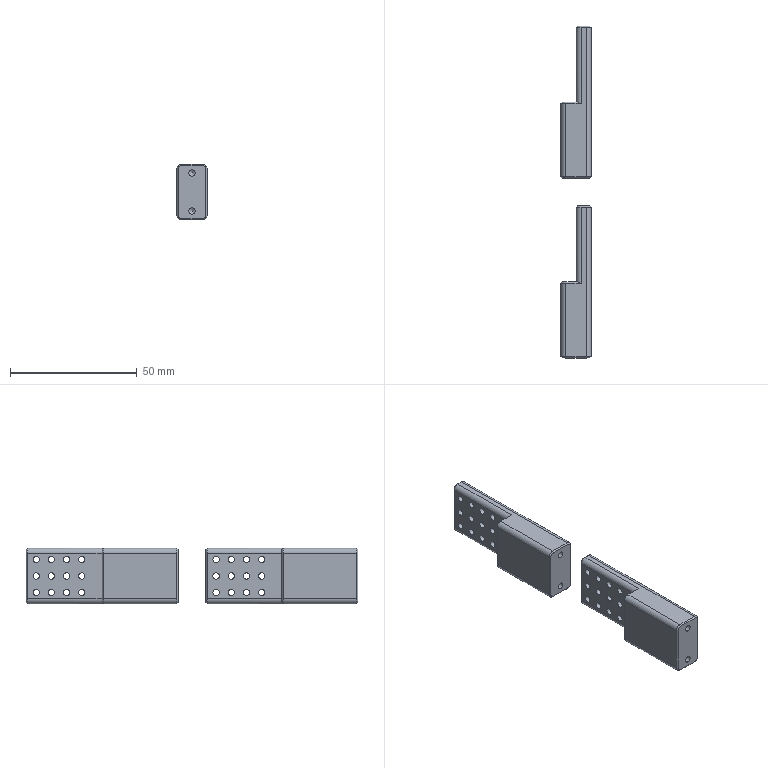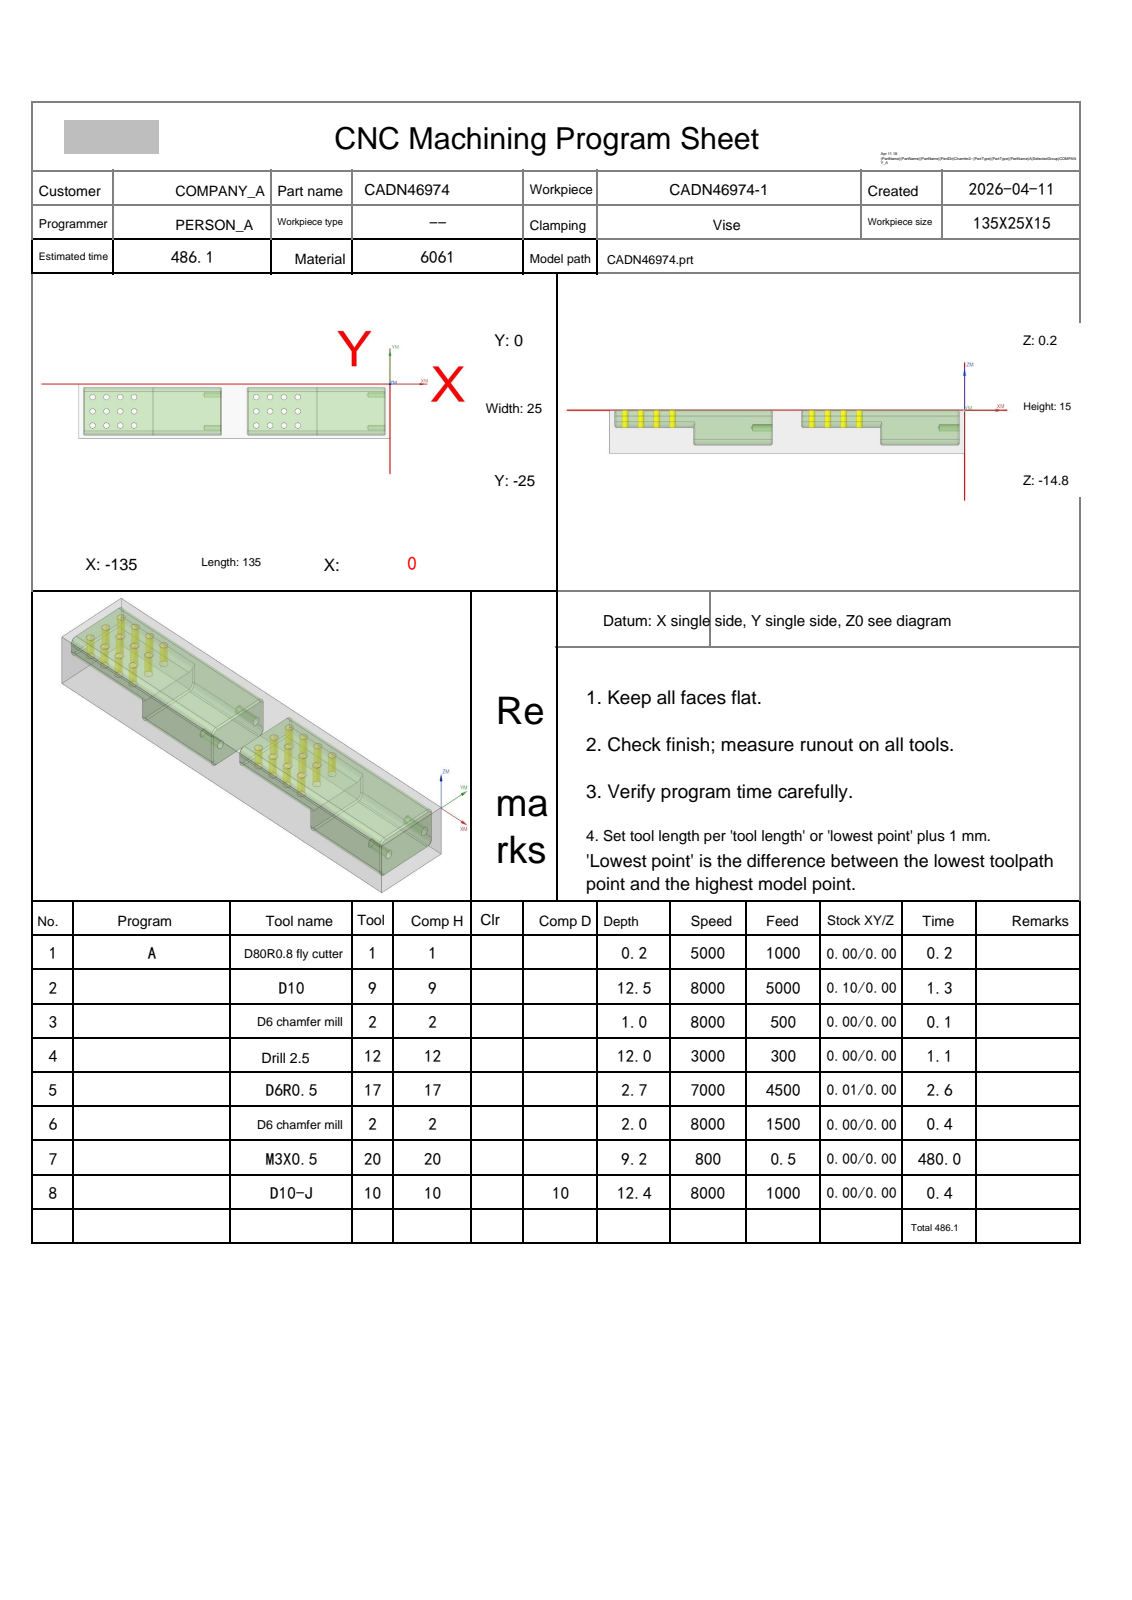NC program | NX | posted by the shop | part box 12 x 131 x 22 mm
Lines 1 to 672 of 2479:
%
O0001
(Machine time: 919.72 MIN)
(===Total Tool:7===)
(T1=D80R0.8 fly cutter D=80.  R=0.8  D-  H01 Z=0.    )
(T9=D10     D=10.  R=0.   D-  H09 Z=-12.3 )
(T2=D6 chamfer mill   D=6.   R=0.   D-  H02 Z=-1.75 )
(T12=drill 2.5  D=2.5  DR_a=118 D-  H12 Z=-11.75)
(T17=D6R0.5 D=6.   R=0.5  D-  H17 Z=-2.5  )
(T20=M3X0.5 D=2.5  DR_a=180 D-  H20 Z=-9.   )
(T10=D10-J  D=10.  R=0.   D10 H10 Z=-12.2 )
G80 G90 G17 G49 G40
G91 G28 Z0
M01
N1 T01 M06
(D80R0.8 fly cutter  D=80. R=0.8 H=01 ce=0.00 di=0.00)
G00 G90 G54 X43. Y-12.5 M03 S5000
G43 H01 Z20.
M08
Z2.
G01 Z0.0 F1000.
X38.
X-173.
X-178.
Z2.
G00 Z20.
G91 G28 Z0.0
M05
M09
G91 G28 Z0.0
M01
N2 T09 M06
(D10  D=10. R=0. H=09 ce=0.10 di=0.00)
G00 G90 G54 X-103. Y-28.6 M03 S8000
G43 H09 Z20.
M08
Z.5
G01 X-132.5 Z.379 F5000.
G02 X-136.106 Y-27.106 Z.362 I0.0 J5.1
G01 X-136.606 Y-26.606 Z.36
G02 X-138.1 Y-23. Z.343 I3.606 J3.606
G01 Y-2. Z.257
G02 X-136.606 Y1.606 Z.24 I5.1 J0.0
G01 X-136.106 Y2.106 Z.238
G02 X-132.5 Y3.6 Z.221 I3.606 J-3.606
G01 X-73.5 Z-.021
G02 X-69.894 Y2.106 Z-.038 I0.0 J-5.1
G01 X-69.394 Y1.606 Z-.04
G02 X-67.9 Y-2. Z-.057 I-3.606 J-3.606
G01 Y-23. Z-.143
G02 X-69.394 Y-26.606 Z-.16 I-5.1 J0.0
G01 X-69.894 Y-27.106 Z-.162
G02 X-73.5 Y-28.6 Z-.179 I-3.606 J3.606
G01 X-132.5 Z-.421
G02 X-136.106 Y-27.106 Z-.438 I0.0 J5.1
G01 X-136.606 Y-26.606 Z-.44
G02 X-138.1 Y-23. Z-.457 I3.606 J3.606
G01 Y-2. Z-.543
G02 X-136.606 Y1.606 Z-.56 I5.1 J0.0
G01 X-136.106 Y2.106 Z-.562
G02 X-132.5 Y3.6 Z-.579 I3.606 J-3.606
G01 X-73.5 Z-.821
G02 X-69.894 Y2.106 Z-.838 I0.0 J-5.1
G01 X-69.394 Y1.606 Z-.84
G02 X-67.9 Y-2. Z-.857 I-3.606 J-3.606
G01 Y-23. Z-.943
G02 X-69.394 Y-26.606 Z-.96 I-5.1 J0.0
G01 X-69.894 Y-27.106 Z-.962
G02 X-73.5 Y-28.6 Z-.979 I-3.606 J3.606
G01 X-132.5 Z-1.221
G02 X-136.106 Y-27.106 Z-1.238 I0.0 J5.1
G01 X-136.606 Y-26.606 Z-1.24
G02 X-138.1 Y-23. Z-1.257 I3.606 J3.606
G01 Y-2. Z-1.343
G02 X-136.606 Y1.606 Z-1.36 I5.1 J0.0
G01 X-136.106 Y2.106 Z-1.362
G02 X-132.5 Y3.6 Z-1.379 I3.606 J-3.606
G01 X-73.5 Z-1.621
G02 X-69.894 Y2.106 Z-1.638 I0.0 J-5.1
G01 X-69.394 Y1.606 Z-1.64
G02 X-67.9 Y-2. Z-1.657 I-3.606 J-3.606
G01 Y-23. Z-1.743
G02 X-69.394 Y-26.606 Z-1.76 I-5.1 J0.0
G01 X-69.894 Y-27.106 Z-1.762
G02 X-73.5 Y-28.6 Z-1.779 I-3.606 J3.606
G01 X-132.5 Z-2.021
G02 X-136.106 Y-27.106 Z-2.038 I0.0 J5.1
G01 X-136.606 Y-26.606 Z-2.04
G02 X-138.1 Y-23. Z-2.057 I3.606 J3.606
G01 Y-2. Z-2.143
G02 X-136.606 Y1.606 Z-2.16 I5.1 J0.0
G01 X-136.106 Y2.106 Z-2.162
G02 X-132.5 Y3.6 Z-2.179 I3.606 J-3.606
G01 X-73.5 Z-2.421
G02 X-69.894 Y2.106 Z-2.438 I0.0 J-5.1
G01 X-69.394 Y1.606 Z-2.44
G02 X-67.9 Y-2. Z-2.457 I-3.606 J-3.606
G01 Y-23. Z-2.543
G02 X-69.394 Y-26.606 Z-2.56 I-5.1 J0.0
G01 X-69.894 Y-27.106 Z-2.562
G02 X-73.5 Y-28.6 Z-2.579 I-3.606 J3.606
G01 X-132.5 Z-2.821
G02 X-136.106 Y-27.106 Z-2.838 I0.0 J5.1
G01 X-136.606 Y-26.606 Z-2.84
G02 X-138.1 Y-23. Z-2.857 I3.606 J3.606
G01 Y-2. Z-2.943
G02 X-136.606 Y1.606 Z-2.96 I5.1 J0.0
G01 X-136.106 Y2.106 Z-2.962
G02 X-132.5 Y3.6 Z-2.979 I3.606 J-3.606
G01 X-73.5 Z-3.221
G02 X-69.894 Y2.106 Z-3.238 I0.0 J-5.1
G01 X-69.394 Y1.606 Z-3.24
G02 X-67.9 Y-2. Z-3.257 I-3.606 J-3.606
G01 Y-23. Z-3.343
G02 X-69.394 Y-26.606 Z-3.36 I-5.1 J0.0
G01 X-69.894 Y-27.106 Z-3.362
G02 X-73.5 Y-28.6 Z-3.379 I-3.606 J3.606
G01 X-132.5 Z-3.621
G02 X-136.106 Y-27.106 Z-3.638 I0.0 J5.1
G01 X-136.606 Y-26.606 Z-3.64
G02 X-138.1 Y-23. Z-3.657 I3.606 J3.606
G01 Y-2. Z-3.743
G02 X-136.606 Y1.606 Z-3.76 I5.1 J0.0
G01 X-136.106 Y2.106 Z-3.762
G02 X-132.5 Y3.6 Z-3.779 I3.606 J-3.606
G01 X-73.5 Z-4.021
G02 X-69.894 Y2.106 Z-4.038 I0.0 J-5.1
G01 X-69.394 Y1.606 Z-4.04
G02 X-67.9 Y-2. Z-4.057 I-3.606 J-3.606
G01 Y-23. Z-4.143
G02 X-69.394 Y-26.606 Z-4.16 I-5.1 J0.0
G01 X-69.894 Y-27.106 Z-4.162
G02 X-73.5 Y-28.6 Z-4.179 I-3.606 J3.606
G01 X-132.5 Z-4.421
G02 X-136.106 Y-27.106 Z-4.438 I0.0 J5.1
G01 X-136.606 Y-26.606 Z-4.44
G02 X-138.1 Y-23. Z-4.457 I3.606 J3.606
G01 Y-2. Z-4.543
G02 X-136.606 Y1.606 Z-4.56 I5.1 J0.0
G01 X-136.106 Y2.106 Z-4.562
G02 X-132.5 Y3.6 Z-4.579 I3.606 J-3.606
G01 X-73.5 Z-4.821
G02 X-69.894 Y2.106 Z-4.838 I0.0 J-5.1
G01 X-69.394 Y1.606 Z-4.84
G02 X-67.9 Y-2. Z-4.857 I-3.606 J-3.606
G01 Y-23. Z-4.943
G02 X-69.394 Y-26.606 Z-4.96 I-5.1 J0.0
G01 X-69.894 Y-27.106 Z-4.962
G02 X-73.5 Y-28.6 Z-4.979 I-3.606 J3.606
G01 X-132.5 Z-5.221
G02 X-136.106 Y-27.106 Z-5.238 I0.0 J5.1
G01 X-136.606 Y-26.606 Z-5.24
G02 X-138.1 Y-23. Z-5.257 I3.606 J3.606
G01 Y-2. Z-5.343
G02 X-136.606 Y1.606 Z-5.36 I5.1 J0.0
G01 X-136.106 Y2.106 Z-5.362
G02 X-132.5 Y3.6 Z-5.379 I3.606 J-3.606
G01 X-73.5 Z-5.621
G02 X-69.894 Y2.106 Z-5.638 I0.0 J-5.1
G01 X-69.394 Y1.606 Z-5.64
G02 X-67.9 Y-2. Z-5.657 I-3.606 J-3.606
G01 Y-23. Z-5.743
G02 X-69.394 Y-26.606 Z-5.76 I-5.1 J0.0
G01 X-69.894 Y-27.106 Z-5.762
G02 X-73.5 Y-28.6 Z-5.779 I-3.606 J3.606
G01 X-132.5 Z-6.021
G02 X-136.106 Y-27.106 Z-6.038 I0.0 J5.1
G01 X-136.606 Y-26.606 Z-6.04
G02 X-138.1 Y-23. Z-6.057 I3.606 J3.606
G01 Y-2. Z-6.143
G02 X-136.606 Y1.606 Z-6.16 I5.1 J0.0
G01 X-136.106 Y2.106 Z-6.162
G02 X-132.5 Y3.6 Z-6.179 I3.606 J-3.606
G01 X-73.5 Z-6.421
G02 X-69.894 Y2.106 Z-6.438 I0.0 J-5.1
G01 X-69.394 Y1.606 Z-6.44
G02 X-67.9 Y-2. Z-6.457 I-3.606 J-3.606
G01 Y-23. Z-6.543
G02 X-69.394 Y-26.606 Z-6.56 I-5.1 J0.0
G01 X-69.894 Y-27.106 Z-6.562
G02 X-73.5 Y-28.6 Z-6.579 I-3.606 J3.606
G01 X-132.5 Z-6.821
G02 X-136.106 Y-27.106 Z-6.838 I0.0 J5.1
G01 X-136.606 Y-26.606 Z-6.84
G02 X-138.1 Y-23. Z-6.857 I3.606 J3.606
G01 Y-2. Z-6.943
G02 X-136.606 Y1.606 Z-6.96 I5.1 J0.0
G01 X-136.106 Y2.106 Z-6.962
G02 X-132.5 Y3.6 Z-6.979 I3.606 J-3.606
G01 X-73.5 Z-7.221
G02 X-69.894 Y2.106 Z-7.238 I0.0 J-5.1
G01 X-69.394 Y1.606 Z-7.24
G02 X-67.9 Y-2. Z-7.257 I-3.606 J-3.606
G01 Y-23. Z-7.343
G02 X-69.394 Y-26.606 Z-7.36 I-5.1 J0.0
G01 X-69.894 Y-27.106 Z-7.362
G02 X-73.5 Y-28.6 Z-7.379 I-3.606 J3.606
G01 X-132.5 Z-7.621
G02 X-136.106 Y-27.106 Z-7.638 I0.0 J5.1
G01 X-136.606 Y-26.606 Z-7.64
G02 X-138.1 Y-23. Z-7.657 I3.606 J3.606
G01 Y-2. Z-7.743
G02 X-136.606 Y1.606 Z-7.76 I5.1 J0.0
G01 X-136.106 Y2.106 Z-7.762
G02 X-132.5 Y3.6 Z-7.779 I3.606 J-3.606
G01 X-73.5 Z-8.021
G02 X-69.894 Y2.106 Z-8.038 I0.0 J-5.1
G01 X-69.394 Y1.606 Z-8.04
G02 X-67.9 Y-2. Z-8.057 I-3.606 J-3.606
G01 Y-23. Z-8.143
G02 X-69.394 Y-26.606 Z-8.16 I-5.1 J0.0
G01 X-69.894 Y-27.106 Z-8.162
G02 X-73.5 Y-28.6 Z-8.179 I-3.606 J3.606
G01 X-132.5 Z-8.421
G02 X-136.106 Y-27.106 Z-8.438 I0.0 J5.1
G01 X-136.606 Y-26.606 Z-8.44
G02 X-138.1 Y-23. Z-8.457 I3.606 J3.606
G01 Y-2. Z-8.543
G02 X-136.606 Y1.606 Z-8.56 I5.1 J0.0
G01 X-136.106 Y2.106 Z-8.562
G02 X-132.5 Y3.6 Z-8.579 I3.606 J-3.606
G01 X-73.5 Z-8.821
G02 X-69.894 Y2.106 Z-8.838 I0.0 J-5.1
G01 X-69.394 Y1.606 Z-8.84
G02 X-67.9 Y-2. Z-8.857 I-3.606 J-3.606
G01 Y-23. Z-8.943
G02 X-69.394 Y-26.606 Z-8.96 I-5.1 J0.0
G01 X-69.894 Y-27.106 Z-8.962
G02 X-73.5 Y-28.6 Z-8.979 I-3.606 J3.606
G01 X-132.5 Z-9.221
G02 X-136.106 Y-27.106 Z-9.238 I0.0 J5.1
G01 X-136.606 Y-26.606 Z-9.24
G02 X-138.1 Y-23. Z-9.257 I3.606 J3.606
G01 Y-2. Z-9.343
G02 X-136.606 Y1.606 Z-9.36 I5.1 J0.0
G01 X-136.106 Y2.106 Z-9.362
G02 X-132.5 Y3.6 Z-9.379 I3.606 J-3.606
G01 X-73.5 Z-9.621
G02 X-69.894 Y2.106 Z-9.638 I0.0 J-5.1
G01 X-69.394 Y1.606 Z-9.64
G02 X-67.9 Y-2. Z-9.657 I-3.606 J-3.606
G01 Y-23. Z-9.743
G02 X-69.394 Y-26.606 Z-9.76 I-5.1 J0.0
G01 X-69.894 Y-27.106 Z-9.762
G02 X-73.5 Y-28.6 Z-9.779 I-3.606 J3.606
G01 X-132.5 Z-10.021
G02 X-136.106 Y-27.106 Z-10.038 I0.0 J5.1
G01 X-136.606 Y-26.606 Z-10.04
G02 X-138.1 Y-23. Z-10.057 I3.606 J3.606
G01 Y-2. Z-10.143
G02 X-136.606 Y1.606 Z-10.16 I5.1 J0.0
G01 X-136.106 Y2.106 Z-10.162
G02 X-132.5 Y3.6 Z-10.179 I3.606 J-3.606
G01 X-73.5 Z-10.421
G02 X-69.894 Y2.106 Z-10.438 I0.0 J-5.1
G01 X-69.394 Y1.606 Z-10.44
G02 X-67.9 Y-2. Z-10.457 I-3.606 J-3.606
G01 Y-23. Z-10.543
G02 X-69.394 Y-26.606 Z-10.56 I-5.1 J0.0
G01 X-69.894 Y-27.106 Z-10.562
G02 X-73.5 Y-28.6 Z-10.579 I-3.606 J3.606
G01 X-132.5 Z-10.821
G02 X-136.106 Y-27.106 Z-10.838 I0.0 J5.1
G01 X-136.606 Y-26.606 Z-10.84
G02 X-138.1 Y-23. Z-10.857 I3.606 J3.606
G01 Y-2. Z-10.943
G02 X-136.606 Y1.606 Z-10.96 I5.1 J0.0
G01 X-136.106 Y2.106 Z-10.962
G02 X-132.5 Y3.6 Z-10.979 I3.606 J-3.606
G01 X-73.5 Z-11.221
G02 X-69.894 Y2.106 Z-11.238 I0.0 J-5.1
G01 X-69.394 Y1.606 Z-11.24
G02 X-67.9 Y-2. Z-11.257 I-3.606 J-3.606
G01 Y-23. Z-11.343
G02 X-69.394 Y-26.606 Z-11.36 I-5.1 J0.0
G01 X-69.894 Y-27.106 Z-11.362
G02 X-73.5 Y-28.6 Z-11.379 I-3.606 J3.606
G01 X-132.5 Z-11.621
G02 X-136.106 Y-27.106 Z-11.638 I0.0 J5.1
G01 X-136.606 Y-26.606 Z-11.64
G02 X-138.1 Y-23. Z-11.657 I3.606 J3.606
G01 Y-2. Z-11.743
G02 X-136.606 Y1.606 Z-11.76 I5.1 J0.0
G01 X-136.106 Y2.106 Z-11.762
G02 X-132.5 Y3.6 Z-11.779 I3.606 J-3.606
G01 X-73.5 Z-12.021
G02 X-69.894 Y2.106 Z-12.038 I0.0 J-5.1
G01 X-69.394 Y1.606 Z-12.04
G02 X-67.9 Y-2. Z-12.057 I-3.606 J-3.606
G01 Y-23. Z-12.143
G02 X-69.394 Y-26.606 Z-12.16 I-5.1 J0.0
G01 X-69.894 Y-27.106 Z-12.162
G02 X-73.5 Y-28.6 Z-12.179 I-3.606 J3.606
G01 X-103. Z-12.3
X-132.5
G02 X-136.106 Y-27.106 I0.0 J5.1
G01 X-136.606 Y-26.606
G02 X-138.1 Y-23. I3.606 J3.606
G01 Y-2.
G02 X-136.606 Y1.606 I5.1 J0.0
G01 X-136.106 Y2.106
G02 X-132.5 Y3.6 I3.606 J-3.606
G01 X-73.5
G02 X-69.894 Y2.106 I0.0 J-5.1
G01 X-69.394 Y1.606
G02 X-67.9 Y-2. I-3.606 J-3.606
G01 Y-23.
G02 X-69.394 Y-26.606 I-5.1 J0.0
G01 X-69.894 Y-27.106
G02 X-73.5 Y-28.6 I-3.606 J3.606
G01 X-103.
X-103.5
Z-11.3
G00 Z20.
X-32.
Z.5
G01 X-61.5 Z.379
G02 X-65.106 Y-27.106 Z.362 I0.0 J5.1
G01 X-65.606 Y-26.606 Z.36
G02 X-67.1 Y-23. Z.343 I3.606 J3.606
G01 Y-2. Z.257
G02 X-65.606 Y1.606 Z.24 I5.1 J0.0
G01 X-65.106 Y2.106 Z.238
G02 X-61.5 Y3.6 Z.221 I3.606 J-3.606
G01 X-2.5 Z-.021
G02 X1.106 Y2.106 Z-.038 I0.0 J-5.1
G01 X1.606 Y1.606 Z-.04
G02 X3.1 Y-2. Z-.057 I-3.606 J-3.606
G01 Y-23. Z-.143
G02 X1.606 Y-26.606 Z-.16 I-5.1 J0.0
G01 X1.106 Y-27.106 Z-.162
G02 X-2.5 Y-28.6 Z-.179 I-3.606 J3.606
G01 X-61.5 Z-.421
G02 X-65.106 Y-27.106 Z-.438 I0.0 J5.1
G01 X-65.606 Y-26.606 Z-.44
G02 X-67.1 Y-23. Z-.457 I3.606 J3.606
G01 Y-2. Z-.543
G02 X-65.606 Y1.606 Z-.56 I5.1 J0.0
G01 X-65.106 Y2.106 Z-.562
G02 X-61.5 Y3.6 Z-.579 I3.606 J-3.606
G01 X-2.5 Z-.821
G02 X1.106 Y2.106 Z-.838 I0.0 J-5.1
G01 X1.606 Y1.606 Z-.84
G02 X3.1 Y-2. Z-.857 I-3.606 J-3.606
G01 Y-23. Z-.943
G02 X1.606 Y-26.606 Z-.96 I-5.1 J0.0
G01 X1.106 Y-27.106 Z-.962
G02 X-2.5 Y-28.6 Z-.979 I-3.606 J3.606
G01 X-61.5 Z-1.221
G02 X-65.106 Y-27.106 Z-1.238 I0.0 J5.1
G01 X-65.606 Y-26.606 Z-1.24
G02 X-67.1 Y-23. Z-1.257 I3.606 J3.606
G01 Y-2. Z-1.343
G02 X-65.606 Y1.606 Z-1.36 I5.1 J0.0
G01 X-65.106 Y2.106 Z-1.362
G02 X-61.5 Y3.6 Z-1.379 I3.606 J-3.606
G01 X-2.5 Z-1.621
G02 X1.106 Y2.106 Z-1.638 I0.0 J-5.1
G01 X1.606 Y1.606 Z-1.64
G02 X3.1 Y-2. Z-1.657 I-3.606 J-3.606
G01 Y-23. Z-1.743
G02 X1.606 Y-26.606 Z-1.76 I-5.1 J0.0
G01 X1.106 Y-27.106 Z-1.762
G02 X-2.5 Y-28.6 Z-1.779 I-3.606 J3.606
G01 X-61.5 Z-2.021
G02 X-65.106 Y-27.106 Z-2.038 I0.0 J5.1
G01 X-65.606 Y-26.606 Z-2.04
G02 X-67.1 Y-23. Z-2.057 I3.606 J3.606
G01 Y-2. Z-2.143
G02 X-65.606 Y1.606 Z-2.16 I5.1 J0.0
G01 X-65.106 Y2.106 Z-2.162
G02 X-61.5 Y3.6 Z-2.179 I3.606 J-3.606
G01 X-2.5 Z-2.421
G02 X1.106 Y2.106 Z-2.438 I0.0 J-5.1
G01 X1.606 Y1.606 Z-2.44
G02 X3.1 Y-2. Z-2.457 I-3.606 J-3.606
G01 Y-23. Z-2.543
G02 X1.606 Y-26.606 Z-2.56 I-5.1 J0.0
G01 X1.106 Y-27.106 Z-2.562
G02 X-2.5 Y-28.6 Z-2.579 I-3.606 J3.606
G01 X-61.5 Z-2.821
G02 X-65.106 Y-27.106 Z-2.838 I0.0 J5.1
G01 X-65.606 Y-26.606 Z-2.84
G02 X-67.1 Y-23. Z-2.857 I3.606 J3.606
G01 Y-2. Z-2.943
G02 X-65.606 Y1.606 Z-2.96 I5.1 J0.0
G01 X-65.106 Y2.106 Z-2.962
G02 X-61.5 Y3.6 Z-2.979 I3.606 J-3.606
G01 X-2.5 Z-3.221
G02 X1.106 Y2.106 Z-3.238 I0.0 J-5.1
G01 X1.606 Y1.606 Z-3.24
G02 X3.1 Y-2. Z-3.257 I-3.606 J-3.606
G01 Y-23. Z-3.343
G02 X1.606 Y-26.606 Z-3.36 I-5.1 J0.0
G01 X1.106 Y-27.106 Z-3.362
G02 X-2.5 Y-28.6 Z-3.379 I-3.606 J3.606
G01 X-61.5 Z-3.621
G02 X-65.106 Y-27.106 Z-3.638 I0.0 J5.1
G01 X-65.606 Y-26.606 Z-3.64
G02 X-67.1 Y-23. Z-3.657 I3.606 J3.606
G01 Y-2. Z-3.743
G02 X-65.606 Y1.606 Z-3.76 I5.1 J0.0
G01 X-65.106 Y2.106 Z-3.762
G02 X-61.5 Y3.6 Z-3.779 I3.606 J-3.606
G01 X-2.5 Z-4.021
G02 X1.106 Y2.106 Z-4.038 I0.0 J-5.1
G01 X1.606 Y1.606 Z-4.04
G02 X3.1 Y-2. Z-4.057 I-3.606 J-3.606
G01 Y-23. Z-4.143
G02 X1.606 Y-26.606 Z-4.16 I-5.1 J0.0
G01 X1.106 Y-27.106 Z-4.162
G02 X-2.5 Y-28.6 Z-4.179 I-3.606 J3.606
G01 X-61.5 Z-4.421
G02 X-65.106 Y-27.106 Z-4.438 I0.0 J5.1
G01 X-65.606 Y-26.606 Z-4.44
G02 X-67.1 Y-23. Z-4.457 I3.606 J3.606
G01 Y-2. Z-4.543
G02 X-65.606 Y1.606 Z-4.56 I5.1 J0.0
G01 X-65.106 Y2.106 Z-4.562
G02 X-61.5 Y3.6 Z-4.579 I3.606 J-3.606
G01 X-2.5 Z-4.821
G02 X1.106 Y2.106 Z-4.838 I0.0 J-5.1
G01 X1.606 Y1.606 Z-4.84
G02 X3.1 Y-2. Z-4.857 I-3.606 J-3.606
G01 Y-23. Z-4.943
G02 X1.606 Y-26.606 Z-4.96 I-5.1 J0.0
G01 X1.106 Y-27.106 Z-4.962
G02 X-2.5 Y-28.6 Z-4.979 I-3.606 J3.606
G01 X-61.5 Z-5.221
G02 X-65.106 Y-27.106 Z-5.238 I0.0 J5.1
G01 X-65.606 Y-26.606 Z-5.24
G02 X-67.1 Y-23. Z-5.257 I3.606 J3.606
G01 Y-2. Z-5.343
G02 X-65.606 Y1.606 Z-5.36 I5.1 J0.0
G01 X-65.106 Y2.106 Z-5.362
G02 X-61.5 Y3.6 Z-5.379 I3.606 J-3.606
G01 X-2.5 Z-5.621
G02 X1.106 Y2.106 Z-5.638 I0.0 J-5.1
G01 X1.606 Y1.606 Z-5.64
G02 X3.1 Y-2. Z-5.657 I-3.606 J-3.606
G01 Y-23. Z-5.743
G02 X1.606 Y-26.606 Z-5.76 I-5.1 J0.0
G01 X1.106 Y-27.106 Z-5.762
G02 X-2.5 Y-28.6 Z-5.779 I-3.606 J3.606
G01 X-61.5 Z-6.021
G02 X-65.106 Y-27.106 Z-6.038 I0.0 J5.1
G01 X-65.606 Y-26.606 Z-6.04
G02 X-67.1 Y-23. Z-6.057 I3.606 J3.606
G01 Y-2. Z-6.143
G02 X-65.606 Y1.606 Z-6.16 I5.1 J0.0
G01 X-65.106 Y2.106 Z-6.162
G02 X-61.5 Y3.6 Z-6.179 I3.606 J-3.606
G01 X-2.5 Z-6.421
G02 X1.106 Y2.106 Z-6.438 I0.0 J-5.1
G01 X1.606 Y1.606 Z-6.44
G02 X3.1 Y-2. Z-6.457 I-3.606 J-3.606
G01 Y-23. Z-6.543
G02 X1.606 Y-26.606 Z-6.56 I-5.1 J0.0
G01 X1.106 Y-27.106 Z-6.562
G02 X-2.5 Y-28.6 Z-6.579 I-3.606 J3.606
G01 X-61.5 Z-6.821
G02 X-65.106 Y-27.106 Z-6.838 I0.0 J5.1
G01 X-65.606 Y-26.606 Z-6.84
G02 X-67.1 Y-23. Z-6.857 I3.606 J3.606
G01 Y-2. Z-6.943
G02 X-65.606 Y1.606 Z-6.96 I5.1 J0.0
G01 X-65.106 Y2.106 Z-6.962
G02 X-61.5 Y3.6 Z-6.979 I3.606 J-3.606
G01 X-2.5 Z-7.221
G02 X1.106 Y2.106 Z-7.238 I0.0 J-5.1
G01 X1.606 Y1.606 Z-7.24
G02 X3.1 Y-2. Z-7.257 I-3.606 J-3.606
G01 Y-23. Z-7.343
G02 X1.606 Y-26.606 Z-7.36 I-5.1 J0.0
G01 X1.106 Y-27.106 Z-7.362
G02 X-2.5 Y-28.6 Z-7.379 I-3.606 J3.606
G01 X-61.5 Z-7.621
G02 X-65.106 Y-27.106 Z-7.638 I0.0 J5.1
G01 X-65.606 Y-26.606 Z-7.64
G02 X-67.1 Y-23. Z-7.657 I3.606 J3.606
G01 Y-2. Z-7.743
G02 X-65.606 Y1.606 Z-7.76 I5.1 J0.0
G01 X-65.106 Y2.106 Z-7.762
G02 X-61.5 Y3.6 Z-7.779 I3.606 J-3.606
G01 X-2.5 Z-8.021
G02 X1.106 Y2.106 Z-8.038 I0.0 J-5.1
G01 X1.606 Y1.606 Z-8.04
G02 X3.1 Y-2. Z-8.057 I-3.606 J-3.606
G01 Y-23. Z-8.143
G02 X1.606 Y-26.606 Z-8.16 I-5.1 J0.0
G01 X1.106 Y-27.106 Z-8.162
G02 X-2.5 Y-28.6 Z-8.179 I-3.606 J3.606
G01 X-61.5 Z-8.421
G02 X-65.106 Y-27.106 Z-8.438 I0.0 J5.1
G01 X-65.606 Y-26.606 Z-8.44
G02 X-67.1 Y-23. Z-8.457 I3.606 J3.606
G01 Y-2. Z-8.543
G02 X-65.606 Y1.606 Z-8.56 I5.1 J0.0
G01 X-65.106 Y2.106 Z-8.562
G02 X-61.5 Y3.6 Z-8.579 I3.606 J-3.606
G01 X-2.5 Z-8.821
G02 X1.106 Y2.106 Z-8.838 I0.0 J-5.1
G01 X1.606 Y1.606 Z-8.84
G02 X3.1 Y-2. Z-8.857 I-3.606 J-3.606
G01 Y-23. Z-8.943
G02 X1.606 Y-26.606 Z-8.96 I-5.1 J0.0
G01 X1.106 Y-27.106 Z-8.962
G02 X-2.5 Y-28.6 Z-8.979 I-3.606 J3.606
G01 X-61.5 Z-9.221
G02 X-65.106 Y-27.106 Z-9.238 I0.0 J5.1
G01 X-65.606 Y-26.606 Z-9.24
G02 X-67.1 Y-23. Z-9.257 I3.606 J3.606
G01 Y-2. Z-9.343
G02 X-65.606 Y1.606 Z-9.36 I5.1 J0.0
G01 X-65.106 Y2.106 Z-9.362
G02 X-61.5 Y3.6 Z-9.379 I3.606 J-3.606
G01 X-2.5 Z-9.621
G02 X1.106 Y2.106 Z-9.638 I0.0 J-5.1
G01 X1.606 Y1.606 Z-9.64
G02 X3.1 Y-2. Z-9.657 I-3.606 J-3.606
G01 Y-23. Z-9.743
G02 X1.606 Y-26.606 Z-9.76 I-5.1 J0.0
G01 X1.106 Y-27.106 Z-9.762
G02 X-2.5 Y-28.6 Z-9.779 I-3.606 J3.606
G01 X-61.5 Z-10.021
G02 X-65.106 Y-27.106 Z-10.038 I0.0 J5.1
G01 X-65.606 Y-26.606 Z-10.04
G02 X-67.1 Y-23. Z-10.057 I3.606 J3.606
G01 Y-2. Z-10.143
G02 X-65.606 Y1.606 Z-10.16 I5.1 J0.0
G01 X-65.106 Y2.106 Z-10.162
G02 X-61.5 Y3.6 Z-10.179 I3.606 J-3.606
G01 X-2.5 Z-10.421
G02 X1.106 Y2.106 Z-10.438 I0.0 J-5.1
G01 X1.606 Y1.606 Z-10.44
G02 X3.1 Y-2. Z-10.457 I-3.606 J-3.606
G01 Y-23. Z-10.543
G02 X1.606 Y-26.606 Z-10.56 I-5.1 J0.0
G01 X1.106 Y-27.106 Z-10.562
G02 X-2.5 Y-28.6 Z-10.579 I-3.606 J3.606
G01 X-61.5 Z-10.821
G02 X-65.106 Y-27.106 Z-10.838 I0.0 J5.1
G01 X-65.606 Y-26.606 Z-10.84
G02 X-67.1 Y-23. Z-10.857 I3.606 J3.606
G01 Y-2. Z-10.943
G02 X-65.606 Y1.606 Z-10.96 I5.1 J0.0
G01 X-65.106 Y2.106 Z-10.962
G02 X-61.5 Y3.6 Z-10.979 I3.606 J-3.606
G01 X-2.5 Z-11.221
G02 X1.106 Y2.106 Z-11.238 I0.0 J-5.1
G01 X1.606 Y1.606 Z-11.24
G02 X3.1 Y-2. Z-11.257 I-3.606 J-3.606
G01 Y-23. Z-11.343
G02 X1.606 Y-26.606 Z-11.36 I-5.1 J0.0
G01 X1.106 Y-27.106 Z-11.362
G02 X-2.5 Y-28.6 Z-11.379 I-3.606 J3.606
G01 X-61.5 Z-11.621
G02 X-65.106 Y-27.106 Z-11.638 I0.0 J5.1
G01 X-65.606 Y-26.606 Z-11.64
G02 X-67.1 Y-23. Z-11.657 I3.606 J3.606
G01 Y-2. Z-11.743
G02 X-65.606 Y1.606 Z-11.76 I5.1 J0.0
G01 X-65.106 Y2.106 Z-11.762
G02 X-61.5 Y3.6 Z-11.779 I3.606 J-3.606
G01 X-2.5 Z-12.021
G02 X1.106 Y2.106 Z-12.038 I0.0 J-5.1
G01 X1.606 Y1.606 Z-12.04
G02 X3.1 Y-2. Z-12.057 I-3.606 J-3.606
G01 Y-23. Z-12.143
G02 X1.606 Y-26.606 Z-12.16 I-5.1 J0.0
G01 X1.106 Y-27.106 Z-12.162
G02 X-2.5 Y-28.6 Z-12.179 I-3.606 J3.606
G01 X-32. Z-12.3
X-61.5
G02 X-65.106 Y-27.106 I0.0 J5.1
G01 X-65.606 Y-26.606
G02 X-67.1 Y-23. I3.606 J3.606
G01 Y-2.
G02 X-65.606 Y1.606 I5.1 J0.0
G01 X-65.106 Y2.106
G02 X-61.5 Y3.6 I3.606 J-3.606
G01 X-2.5
G02 X1.106 Y2.106 I0.0 J-5.1
G01 X1.606 Y1.606
G02 X3.1 Y-2. I-3.606 J-3.606
G01 Y-23.
G02 X1.606 Y-26.606 I-5.1 J0.0
G01 X1.106 Y-27.106
G02 X-2.5 Y-28.6 I-3.606 J3.606
G01 X-32.
X-32.5
Z-11.3
G00 Z20.
G91 G28 Z0.0
M05
M09
G91 G28 Z0.0
M01
N3 T02 M06
(D6 chamfer mill  D=6. R=0. H=02 ce=0.00 di=0.00)
G00 G90 G54 X-40. Y-19. M03 S8000
G43 H02 Z20.
M08
G98 G81 X-40. Y-19. Z-.8 R1. F500.
X-46.
X-52.
X-58.
Y-12.5
X-52.
X-46.
X-40.
Y-6.
X-46.
X-52.
X-58.
X-111.
X-117.
X-123.
X-129.
Y-12.5
X-123.
X-117.
X-111.
Y-19.
X-117.
X-123.
X-129.
G80
G00 Z20.
G91 G28 Z0.0
M05
M09
G91 G28 Z0.0
M01
N4 T12 M06
(drill 2.5 D=2.5 DR_a=118 H=12)
G00 G90 G54 X-40. Y-19. M03 S3000
G43 H12 Z20.
M08
G98 G83 X-40. Y-19. Z-11.751 R1. F300. Q2.
X-46.
X-52.
X-58.
Y-12.5
X-52.
X-46.
X-40.
Y-6.
X-46.
X-52.
X-58.
X-111.
X-117.
X-123.
X-129.
Y-12.5
X-123.
X-117.
X-111.
Y-19.
X-117.
X-123.
X-129.
G80
G00 Z20.
G91 G28 Z0.0
M05
M09
G91 G28 Z0.0
M01